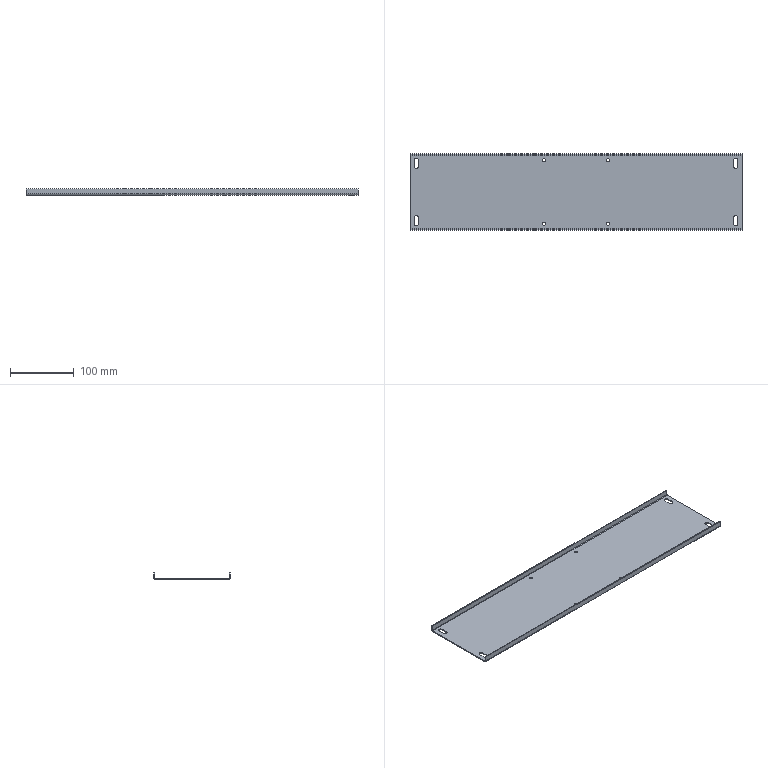Part | STEP file | Guide wheel mechanism revised.sldasm-Part-314 | 1 solid | 46 faces | box 520 x 120 x 10 mm | volume 105158 mm3 | plane 26 | cylinder 20 | commonest cylinder face diameters 5 x8 6.5 x8 1.473 x2 4.473 x2
STEP:
#1=CARTESIAN_POINT('',(-52.5,-50.,-1.5));
#2=VERTEX_POINT('',#1);
#3=CARTESIAN_POINT('',(-47.5,-50.,-1.5));
#4=VERTEX_POINT('',#3);
#5=CARTESIAN_POINT('',(-50.,-50.,-1.5));
#6=DIRECTION('',(0.,0.,1.));
#7=DIRECTION('',(1.,0.,0.));
#8=AXIS2_PLACEMENT_3D('',#5,#6,#7);
#9=CIRCLE('',#8,2.5);
#10=EDGE_CURVE('',#2,#4,#9,.T.);
#11=ORIENTED_EDGE('',*,*,#10,.F.);
#12=CARTESIAN_POINT('',(-52.5,-50.,0.));
#13=VERTEX_POINT('',#12);
#14=CARTESIAN_POINT('',(-52.5,-50.,0.));
#15=DIRECTION('',(0.,0.,1.));
#16=VECTOR('',#15,1000.);
#17=LINE('',#14,#16);
#18=EDGE_CURVE('',#2,#13,#17,.T.);
#19=ORIENTED_EDGE('',*,*,#18,.T.);
#20=CARTESIAN_POINT('',(-47.5,-50.,0.));
#21=VERTEX_POINT('',#20);
#22=CARTESIAN_POINT('',(-50.,-50.,0.));
#23=DIRECTION('',(0.,0.,1.));
#24=DIRECTION('',(1.,0.,0.));
#25=AXIS2_PLACEMENT_3D('',#22,#23,#24);
#26=CIRCLE('',#25,2.5);
#27=EDGE_CURVE('',#13,#21,#26,.T.);
#28=ORIENTED_EDGE('',*,*,#27,.T.);
#29=CARTESIAN_POINT('',(-47.5,-50.,0.));
#30=DIRECTION('',(0.,0.,1.));
#31=VECTOR('',#30,1000.);
#32=LINE('',#29,#31);
#33=EDGE_CURVE('',#4,#21,#32,.T.);
#34=ORIENTED_EDGE('',*,*,#33,.F.);
#35=EDGE_LOOP('',(#11,#19,#28,#34));
#36=FACE_OUTER_BOUND('',#35,.T.);
#37=CARTESIAN_POINT('',(-50.,-50.,0.));
#38=DIRECTION('',(0.,0.,1.));
#39=DIRECTION('',(1.,0.,0.));
#40=AXIS2_PLACEMENT_3D('',#37,#38,#39);
#41=CYLINDRICAL_SURFACE('',#40,2.5);
#42=ADVANCED_FACE('',(#36),#41,.F.);
#43=CARTESIAN_POINT('',(-52.5,50.,-1.5));
#44=VERTEX_POINT('',#43);
#45=CARTESIAN_POINT('',(-47.5,50.,-1.5));
#46=VERTEX_POINT('',#45);
#47=CARTESIAN_POINT('',(-50.,50.,-1.5));
#48=DIRECTION('',(0.,0.,1.));
#49=DIRECTION('',(1.,0.,0.));
#50=AXIS2_PLACEMENT_3D('',#47,#48,#49);
#51=CIRCLE('',#50,2.5);
#52=EDGE_CURVE('',#44,#46,#51,.T.);
#53=ORIENTED_EDGE('',*,*,#52,.F.);
#54=CARTESIAN_POINT('',(-52.5,50.,0.));
#55=VERTEX_POINT('',#54);
#56=CARTESIAN_POINT('',(-52.5,50.,0.));
#57=DIRECTION('',(0.,0.,1.));
#58=VECTOR('',#57,1000.);
#59=LINE('',#56,#58);
#60=EDGE_CURVE('',#44,#55,#59,.T.);
#61=ORIENTED_EDGE('',*,*,#60,.T.);
#62=CARTESIAN_POINT('',(-47.5,50.,0.));
#63=VERTEX_POINT('',#62);
#64=CARTESIAN_POINT('',(-50.,50.,0.));
#65=DIRECTION('',(0.,0.,1.));
#66=DIRECTION('',(1.,0.,0.));
#67=AXIS2_PLACEMENT_3D('',#64,#65,#66);
#68=CIRCLE('',#67,2.5);
#69=EDGE_CURVE('',#55,#63,#68,.T.);
#70=ORIENTED_EDGE('',*,*,#69,.T.);
#71=CARTESIAN_POINT('',(-47.5,50.,0.));
#72=DIRECTION('',(0.,0.,1.));
#73=VECTOR('',#72,1000.);
#74=LINE('',#71,#73);
#75=EDGE_CURVE('',#46,#63,#74,.T.);
#76=ORIENTED_EDGE('',*,*,#75,.F.);
#77=EDGE_LOOP('',(#53,#61,#70,#76));
#78=FACE_OUTER_BOUND('',#77,.T.);
#79=CARTESIAN_POINT('',(-50.,50.,0.));
#80=DIRECTION('',(0.,0.,1.));
#81=DIRECTION('',(1.,0.,0.));
#82=AXIS2_PLACEMENT_3D('',#79,#80,#81);
#83=CYLINDRICAL_SURFACE('',#82,2.5);
#84=ADVANCED_FACE('',(#78),#83,.F.);
#85=CARTESIAN_POINT('',(47.5,-50.,-1.5));
#86=VERTEX_POINT('',#85);
#87=CARTESIAN_POINT('',(52.5,-50.,-1.5));
#88=VERTEX_POINT('',#87);
#89=CARTESIAN_POINT('',(50.,-50.,-1.5));
#90=DIRECTION('',(0.,0.,1.));
#91=DIRECTION('',(1.,0.,0.));
#92=AXIS2_PLACEMENT_3D('',#89,#90,#91);
#93=CIRCLE('',#92,2.5);
#94=EDGE_CURVE('',#86,#88,#93,.T.);
#95=ORIENTED_EDGE('',*,*,#94,.F.);
#96=CARTESIAN_POINT('',(47.5,-50.,0.));
#97=VERTEX_POINT('',#96);
#98=CARTESIAN_POINT('',(47.5,-50.,0.));
#99=DIRECTION('',(0.,0.,1.));
#100=VECTOR('',#99,1000.);
#101=LINE('',#98,#100);
#102=EDGE_CURVE('',#86,#97,#101,.T.);
#103=ORIENTED_EDGE('',*,*,#102,.T.);
#104=CARTESIAN_POINT('',(52.5,-50.,0.));
#105=VERTEX_POINT('',#104);
#106=CARTESIAN_POINT('',(50.,-50.,0.));
#107=DIRECTION('',(0.,0.,1.));
#108=DIRECTION('',(1.,0.,0.));
#109=AXIS2_PLACEMENT_3D('',#106,#107,#108);
#110=CIRCLE('',#109,2.5);
#111=EDGE_CURVE('',#97,#105,#110,.T.);
#112=ORIENTED_EDGE('',*,*,#111,.T.);
#113=CARTESIAN_POINT('',(52.5,-50.,0.));
#114=DIRECTION('',(0.,0.,1.));
#115=VECTOR('',#114,1000.);
#116=LINE('',#113,#115);
#117=EDGE_CURVE('',#88,#105,#116,.T.);
#118=ORIENTED_EDGE('',*,*,#117,.F.);
#119=EDGE_LOOP('',(#95,#103,#112,#118));
#120=FACE_OUTER_BOUND('',#119,.T.);
#121=CARTESIAN_POINT('',(50.,-50.,0.));
#122=DIRECTION('',(0.,0.,1.));
#123=DIRECTION('',(1.,0.,0.));
#124=AXIS2_PLACEMENT_3D('',#121,#122,#123);
#125=CYLINDRICAL_SURFACE('',#124,2.5);
#126=ADVANCED_FACE('',(#120),#125,.F.);
#127=CARTESIAN_POINT('',(47.5,50.,-1.5));
#128=VERTEX_POINT('',#127);
#129=CARTESIAN_POINT('',(52.5,50.,-1.5));
#130=VERTEX_POINT('',#129);
#131=CARTESIAN_POINT('',(50.,50.,-1.5));
#132=DIRECTION('',(0.,0.,1.));
#133=DIRECTION('',(1.,0.,0.));
#134=AXIS2_PLACEMENT_3D('',#131,#132,#133);
#135=CIRCLE('',#134,2.5);
#136=EDGE_CURVE('',#128,#130,#135,.T.);
#137=ORIENTED_EDGE('',*,*,#136,.F.);
#138=CARTESIAN_POINT('',(47.5,50.,0.));
#139=VERTEX_POINT('',#138);
#140=CARTESIAN_POINT('',(47.5,50.,0.));
#141=DIRECTION('',(0.,0.,1.));
#142=VECTOR('',#141,1000.);
#143=LINE('',#140,#142);
#144=EDGE_CURVE('',#128,#139,#143,.T.);
#145=ORIENTED_EDGE('',*,*,#144,.T.);
#146=CARTESIAN_POINT('',(52.5,50.,0.));
#147=VERTEX_POINT('',#146);
#148=CARTESIAN_POINT('',(50.,50.,0.));
#149=DIRECTION('',(0.,0.,1.));
#150=DIRECTION('',(1.,0.,0.));
#151=AXIS2_PLACEMENT_3D('',#148,#149,#150);
#152=CIRCLE('',#151,2.5);
#153=EDGE_CURVE('',#139,#147,#152,.T.);
#154=ORIENTED_EDGE('',*,*,#153,.T.);
#155=CARTESIAN_POINT('',(52.5,50.,0.));
#156=DIRECTION('',(0.,0.,1.));
#157=VECTOR('',#156,1000.);
#158=LINE('',#155,#157);
#159=EDGE_CURVE('',#130,#147,#158,.T.);
#160=ORIENTED_EDGE('',*,*,#159,.F.);
#161=EDGE_LOOP('',(#137,#145,#154,#160));
#162=FACE_OUTER_BOUND('',#161,.T.);
#163=CARTESIAN_POINT('',(50.,50.,0.));
#164=DIRECTION('',(0.,0.,1.));
#165=DIRECTION('',(1.,0.,0.));
#166=AXIS2_PLACEMENT_3D('',#163,#164,#165);
#167=CYLINDRICAL_SURFACE('',#166,2.5);
#168=ADVANCED_FACE('',(#162),#167,.F.);
#169=CARTESIAN_POINT('',(-246.75,50.,-1.5));
#170=VERTEX_POINT('',#169);
#171=CARTESIAN_POINT('',(-246.75,40.,-1.5));
#172=VERTEX_POINT('',#171);
#173=CARTESIAN_POINT('',(-246.75,50.,-1.5));
#174=DIRECTION('',(0.,-1.,0.));
#175=VECTOR('',#174,1000.);
#176=LINE('',#173,#175);
#177=EDGE_CURVE('',#170,#172,#176,.T.);
#178=ORIENTED_EDGE('',*,*,#177,.F.);
#179=CARTESIAN_POINT('',(-253.25,50.,-1.5));
#180=VERTEX_POINT('',#179);
#181=CARTESIAN_POINT('',(-250.,50.,-1.5));
#182=DIRECTION('',(0.,0.,-1.));
#183=DIRECTION('',(-1.,0.,0.));
#184=AXIS2_PLACEMENT_3D('',#181,#182,#183);
#185=CIRCLE('',#184,3.25);
#186=EDGE_CURVE('',#180,#170,#185,.T.);
#187=ORIENTED_EDGE('',*,*,#186,.F.);
#188=CARTESIAN_POINT('',(-253.25,40.,-1.5));
#189=VERTEX_POINT('',#188);
#190=CARTESIAN_POINT('',(-253.25,50.,-1.5));
#191=DIRECTION('',(0.,1.,0.));
#192=VECTOR('',#191,1000.);
#193=LINE('',#190,#192);
#194=EDGE_CURVE('',#189,#180,#193,.T.);
#195=ORIENTED_EDGE('',*,*,#194,.F.);
#196=CARTESIAN_POINT('',(-250.,40.,-1.5));
#197=DIRECTION('',(0.,0.,-1.));
#198=DIRECTION('',(-1.,0.,0.));
#199=AXIS2_PLACEMENT_3D('',#196,#197,#198);
#200=CIRCLE('',#199,3.25);
#201=EDGE_CURVE('',#172,#189,#200,.T.);
#202=ORIENTED_EDGE('',*,*,#201,.F.);
#203=EDGE_LOOP('',(#178,#187,#195,#202));
#204=FACE_BOUND('',#203,.T.);
#205=CARTESIAN_POINT('',(253.25,50.,-1.5));
#206=VERTEX_POINT('',#205);
#207=CARTESIAN_POINT('',(253.25,40.,-1.5));
#208=VERTEX_POINT('',#207);
#209=CARTESIAN_POINT('',(253.25,50.,-1.5));
#210=DIRECTION('',(0.,-1.,0.));
#211=VECTOR('',#210,1000.);
#212=LINE('',#209,#211);
#213=EDGE_CURVE('',#206,#208,#212,.T.);
#214=ORIENTED_EDGE('',*,*,#213,.F.);
#215=CARTESIAN_POINT('',(246.75,50.,-1.5));
#216=VERTEX_POINT('',#215);
#217=CARTESIAN_POINT('',(250.,50.,-1.5));
#218=DIRECTION('',(0.,0.,-1.));
#219=DIRECTION('',(-1.,0.,0.));
#220=AXIS2_PLACEMENT_3D('',#217,#218,#219);
#221=CIRCLE('',#220,3.25);
#222=EDGE_CURVE('',#216,#206,#221,.T.);
#223=ORIENTED_EDGE('',*,*,#222,.F.);
#224=CARTESIAN_POINT('',(246.75,40.,-1.5));
#225=VERTEX_POINT('',#224);
#226=CARTESIAN_POINT('',(246.75,50.,-1.5));
#227=DIRECTION('',(0.,1.,0.));
#228=VECTOR('',#227,1000.);
#229=LINE('',#226,#228);
#230=EDGE_CURVE('',#225,#216,#229,.T.);
#231=ORIENTED_EDGE('',*,*,#230,.F.);
#232=CARTESIAN_POINT('',(250.,40.,-1.5));
#233=DIRECTION('',(0.,0.,-1.));
#234=DIRECTION('',(-1.,0.,0.));
#235=AXIS2_PLACEMENT_3D('',#232,#233,#234);
#236=CIRCLE('',#235,3.25);
#237=EDGE_CURVE('',#208,#225,#236,.T.);
#238=ORIENTED_EDGE('',*,*,#237,.F.);
#239=EDGE_LOOP('',(#214,#223,#231,#238));
#240=FACE_BOUND('',#239,.T.);
#241=CARTESIAN_POINT('',(-50.,-50.,-1.5));
#242=DIRECTION('',(0.,0.,1.));
#243=DIRECTION('',(1.,0.,0.));
#244=AXIS2_PLACEMENT_3D('',#241,#242,#243);
#245=CIRCLE('',#244,2.5);
#246=EDGE_CURVE('',#4,#2,#245,.T.);
#247=ORIENTED_EDGE('',*,*,#246,.T.);
#248=ORIENTED_EDGE('',*,*,#10,.T.);
#249=EDGE_LOOP('',(#247,#248));
#250=FACE_BOUND('',#249,.T.);
#251=CARTESIAN_POINT('',(-50.,50.,-1.5));
#252=DIRECTION('',(0.,0.,1.));
#253=DIRECTION('',(1.,0.,0.));
#254=AXIS2_PLACEMENT_3D('',#251,#252,#253);
#255=CIRCLE('',#254,2.5);
#256=EDGE_CURVE('',#46,#44,#255,.T.);
#257=ORIENTED_EDGE('',*,*,#256,.T.);
#258=ORIENTED_EDGE('',*,*,#52,.T.);
#259=EDGE_LOOP('',(#257,#258));
#260=FACE_BOUND('',#259,.T.);
#261=CARTESIAN_POINT('',(50.,-50.,-1.5));
#262=DIRECTION('',(0.,0.,1.));
#263=DIRECTION('',(1.,0.,0.));
#264=AXIS2_PLACEMENT_3D('',#261,#262,#263);
#265=CIRCLE('',#264,2.5);
#266=EDGE_CURVE('',#88,#86,#265,.T.);
#267=ORIENTED_EDGE('',*,*,#266,.T.);
#268=ORIENTED_EDGE('',*,*,#94,.T.);
#269=EDGE_LOOP('',(#267,#268));
#270=FACE_BOUND('',#269,.T.);
#271=CARTESIAN_POINT('',(50.,50.,-1.5));
#272=DIRECTION('',(0.,0.,1.));
#273=DIRECTION('',(1.,0.,0.));
#274=AXIS2_PLACEMENT_3D('',#271,#272,#273);
#275=CIRCLE('',#274,2.5);
#276=EDGE_CURVE('',#130,#128,#275,.T.);
#277=ORIENTED_EDGE('',*,*,#276,.T.);
#278=ORIENTED_EDGE('',*,*,#136,.T.);
#279=EDGE_LOOP('',(#277,#278));
#280=FACE_BOUND('',#279,.T.);
#281=CARTESIAN_POINT('',(260.,-57.763,-1.5));
#282=VERTEX_POINT('',#281);
#283=CARTESIAN_POINT('',(-260.,-57.763,-1.5));
#284=VERTEX_POINT('',#283);
#285=CARTESIAN_POINT('',(260.,-57.763,-1.5));
#286=DIRECTION('',(-1.,0.,0.));
#287=VECTOR('',#286,1000.);
#288=LINE('',#285,#287);
#289=EDGE_CURVE('',#282,#284,#288,.T.);
#290=ORIENTED_EDGE('',*,*,#289,.T.);
#291=CARTESIAN_POINT('',(-260.,57.763,-1.5));
#292=VERTEX_POINT('',#291);
#293=CARTESIAN_POINT('',(-260.,60.,-1.5));
#294=DIRECTION('',(0.,-1.,0.));
#295=VECTOR('',#294,1000.);
#296=LINE('',#293,#295);
#297=EDGE_CURVE('',#292,#284,#296,.T.);
#298=ORIENTED_EDGE('',*,*,#297,.F.);
#299=CARTESIAN_POINT('',(260.,57.763,-1.5));
#300=VERTEX_POINT('',#299);
#301=CARTESIAN_POINT('',(-260.,57.763,-1.5));
#302=DIRECTION('',(1.,0.,0.));
#303=VECTOR('',#302,1000.);
#304=LINE('',#301,#303);
#305=EDGE_CURVE('',#292,#300,#304,.T.);
#306=ORIENTED_EDGE('',*,*,#305,.T.);
#307=CARTESIAN_POINT('',(260.,60.,-1.5));
#308=DIRECTION('',(0.,1.,0.));
#309=VECTOR('',#308,1000.);
#310=LINE('',#307,#309);
#311=EDGE_CURVE('',#282,#300,#310,.T.);
#312=ORIENTED_EDGE('',*,*,#311,.F.);
#313=EDGE_LOOP('',(#290,#298,#306,#312));
#314=FACE_OUTER_BOUND('',#313,.T.);
#315=CARTESIAN_POINT('',(246.75,-40.,-1.5));
#316=VERTEX_POINT('',#315);
#317=CARTESIAN_POINT('',(253.25,-40.,-1.5));
#318=VERTEX_POINT('',#317);
#319=CARTESIAN_POINT('',(250.,-40.,-1.5));
#320=DIRECTION('',(0.,0.,-1.));
#321=DIRECTION('',(-1.,0.,0.));
#322=AXIS2_PLACEMENT_3D('',#319,#320,#321);
#323=CIRCLE('',#322,3.25);
#324=EDGE_CURVE('',#316,#318,#323,.T.);
#325=ORIENTED_EDGE('',*,*,#324,.F.);
#326=CARTESIAN_POINT('',(246.75,-50.,-1.5));
#327=VERTEX_POINT('',#326);
#328=CARTESIAN_POINT('',(246.75,-40.,-1.5));
#329=DIRECTION('',(0.,1.,0.));
#330=VECTOR('',#329,1000.);
#331=LINE('',#328,#330);
#332=EDGE_CURVE('',#327,#316,#331,.T.);
#333=ORIENTED_EDGE('',*,*,#332,.F.);
#334=CARTESIAN_POINT('',(253.25,-50.,-1.5));
#335=VERTEX_POINT('',#334);
#336=CARTESIAN_POINT('',(250.,-50.,-1.5));
#337=DIRECTION('',(0.,0.,-1.));
#338=DIRECTION('',(-1.,0.,0.));
#339=AXIS2_PLACEMENT_3D('',#336,#337,#338);
#340=CIRCLE('',#339,3.25);
#341=EDGE_CURVE('',#335,#327,#340,.T.);
#342=ORIENTED_EDGE('',*,*,#341,.F.);
#343=CARTESIAN_POINT('',(253.25,-40.,-1.5));
#344=DIRECTION('',(0.,-1.,0.));
#345=VECTOR('',#344,1000.);
#346=LINE('',#343,#345);
#347=EDGE_CURVE('',#318,#335,#346,.T.);
#348=ORIENTED_EDGE('',*,*,#347,.F.);
#349=EDGE_LOOP('',(#325,#333,#342,#348));
#350=FACE_BOUND('',#349,.T.);
#351=CARTESIAN_POINT('',(-253.25,-40.,-1.5));
#352=VERTEX_POINT('',#351);
#353=CARTESIAN_POINT('',(-246.75,-40.,-1.5));
#354=VERTEX_POINT('',#353);
#355=CARTESIAN_POINT('',(-250.,-40.,-1.5));
#356=DIRECTION('',(0.,0.,-1.));
#357=DIRECTION('',(-1.,0.,0.));
#358=AXIS2_PLACEMENT_3D('',#355,#356,#357);
#359=CIRCLE('',#358,3.25);
#360=EDGE_CURVE('',#352,#354,#359,.T.);
#361=ORIENTED_EDGE('',*,*,#360,.F.);
#362=CARTESIAN_POINT('',(-253.25,-50.,-1.5));
#363=VERTEX_POINT('',#362);
#364=CARTESIAN_POINT('',(-253.25,-40.,-1.5));
#365=DIRECTION('',(0.,1.,0.));
#366=VECTOR('',#365,1000.);
#367=LINE('',#364,#366);
#368=EDGE_CURVE('',#363,#352,#367,.T.);
#369=ORIENTED_EDGE('',*,*,#368,.F.);
#370=CARTESIAN_POINT('',(-246.75,-50.,-1.5));
#371=VERTEX_POINT('',#370);
#372=CARTESIAN_POINT('',(-250.,-50.,-1.5));
#373=DIRECTION('',(0.,0.,-1.));
#374=DIRECTION('',(-1.,0.,0.));
#375=AXIS2_PLACEMENT_3D('',#372,#373,#374);
#376=CIRCLE('',#375,3.25);
#377=EDGE_CURVE('',#371,#363,#376,.T.);
#378=ORIENTED_EDGE('',*,*,#377,.F.);
#379=CARTESIAN_POINT('',(-246.75,-40.,-1.5));
#380=DIRECTION('',(0.,-1.,0.));
#381=VECTOR('',#380,1000.);
#382=LINE('',#379,#381);
#383=EDGE_CURVE('',#354,#371,#382,.T.);
#384=ORIENTED_EDGE('',*,*,#383,.F.);
#385=EDGE_LOOP('',(#361,#369,#378,#384));
#386=FACE_BOUND('',#385,.T.);
#387=CARTESIAN_POINT('',(260.,-60.,-1.5));
#388=DIRECTION('',(0.,0.,1.));
#389=DIRECTION('',(1.,0.,0.));
#390=AXIS2_PLACEMENT_3D('',#387,#388,#389);
#391=PLANE('',#390);
#392=ADVANCED_FACE('',(#204,#240,#250,#260,#270,#280,#314,#350,#386),#391,.F.);
#393=CARTESIAN_POINT('',(-253.25,50.,0.));
#394=VERTEX_POINT('',#393);
#395=CARTESIAN_POINT('',(-246.75,50.,0.));
#396=VERTEX_POINT('',#395);
#397=CARTESIAN_POINT('',(-250.,50.,0.));
#398=DIRECTION('',(0.,0.,-1.));
#399=DIRECTION('',(-1.,0.,0.));
#400=AXIS2_PLACEMENT_3D('',#397,#398,#399);
#401=CIRCLE('',#400,3.25);
#402=EDGE_CURVE('',#394,#396,#401,.T.);
#403=ORIENTED_EDGE('',*,*,#402,.T.);
#404=CARTESIAN_POINT('',(-246.75,40.,0.));
#405=VERTEX_POINT('',#404);
#406=CARTESIAN_POINT('',(-246.75,50.,0.));
#407=DIRECTION('',(0.,-1.,0.));
#408=VECTOR('',#407,1000.);
#409=LINE('',#406,#408);
#410=EDGE_CURVE('',#396,#405,#409,.T.);
#411=ORIENTED_EDGE('',*,*,#410,.T.);
#412=CARTESIAN_POINT('',(-253.25,40.,0.));
#413=VERTEX_POINT('',#412);
#414=CARTESIAN_POINT('',(-250.,40.,0.));
#415=DIRECTION('',(0.,0.,-1.));
#416=DIRECTION('',(-1.,0.,0.));
#417=AXIS2_PLACEMENT_3D('',#414,#415,#416);
#418=CIRCLE('',#417,3.25);
#419=EDGE_CURVE('',#405,#413,#418,.T.);
#420=ORIENTED_EDGE('',*,*,#419,.T.);
#421=CARTESIAN_POINT('',(-253.25,50.,0.));
#422=DIRECTION('',(0.,1.,0.));
#423=VECTOR('',#422,1000.);
#424=LINE('',#421,#423);
#425=EDGE_CURVE('',#413,#394,#424,.T.);
#426=ORIENTED_EDGE('',*,*,#425,.T.);
#427=EDGE_LOOP('',(#403,#411,#420,#426));
#428=FACE_BOUND('',#427,.T.);
#429=CARTESIAN_POINT('',(246.75,50.,0.));
#430=VERTEX_POINT('',#429);
#431=CARTESIAN_POINT('',(253.25,50.,0.));
#432=VERTEX_POINT('',#431);
#433=CARTESIAN_POINT('',(250.,50.,0.));
#434=DIRECTION('',(0.,0.,-1.));
#435=DIRECTION('',(-1.,0.,0.));
#436=AXIS2_PLACEMENT_3D('',#433,#434,#435);
#437=CIRCLE('',#436,3.25);
#438=EDGE_CURVE('',#430,#432,#437,.T.);
#439=ORIENTED_EDGE('',*,*,#438,.T.);
#440=CARTESIAN_POINT('',(253.25,40.,0.));
#441=VERTEX_POINT('',#440);
#442=CARTESIAN_POINT('',(253.25,50.,0.));
#443=DIRECTION('',(0.,-1.,0.));
#444=VECTOR('',#443,1000.);
#445=LINE('',#442,#444);
#446=EDGE_CURVE('',#432,#441,#445,.T.);
#447=ORIENTED_EDGE('',*,*,#446,.T.);
#448=CARTESIAN_POINT('',(246.75,40.,0.));
#449=VERTEX_POINT('',#448);
#450=CARTESIAN_POINT('',(250.,40.,0.));
#451=DIRECTION('',(0.,0.,-1.));
#452=DIRECTION('',(-1.,0.,0.));
#453=AXIS2_PLACEMENT_3D('',#450,#451,#452);
#454=CIRCLE('',#453,3.25);
#455=EDGE_CURVE('',#441,#449,#454,.T.);
#456=ORIENTED_EDGE('',*,*,#455,.T.);
#457=CARTESIAN_POINT('',(246.75,50.,0.));
#458=DIRECTION('',(0.,1.,0.));
#459=VECTOR('',#458,1000.);
#460=LINE('',#457,#459);
#461=EDGE_CURVE('',#449,#430,#460,.T.);
#462=ORIENTED_EDGE('',*,*,#461,.T.);
#463=EDGE_LOOP('',(#439,#447,#456,#462));
#464=FACE_BOUND('',#463,.T.);
#465=CARTESIAN_POINT('',(-50.,-50.,0.));
#466=DIRECTION('',(0.,0.,1.));
#467=DIRECTION('',(1.,0.,0.));
#468=AXIS2_PLACEMENT_3D('',#465,#466,#467);
#469=CIRCLE('',#468,2.5);
#470=EDGE_CURVE('',#21,#13,#469,.T.);
#471=ORIENTED_EDGE('',*,*,#470,.F.);
#472=ORIENTED_EDGE('',*,*,#27,.F.);
#473=EDGE_LOOP('',(#471,#472));
#474=FACE_BOUND('',#473,.T.);
#475=CARTESIAN_POINT('',(-50.,50.,0.));
#476=DIRECTION('',(0.,0.,1.));
#477=DIRECTION('',(1.,0.,0.));
#478=AXIS2_PLACEMENT_3D('',#475,#476,#477);
#479=CIRCLE('',#478,2.5);
#480=EDGE_CURVE('',#63,#55,#479,.T.);
#481=ORIENTED_EDGE('',*,*,#480,.F.);
#482=ORIENTED_EDGE('',*,*,#69,.F.);
#483=EDGE_LOOP('',(#481,#482));
#484=FACE_BOUND('',#483,.T.);
#485=CARTESIAN_POINT('',(50.,-50.,0.));
#486=DIRECTION('',(0.,0.,1.));
#487=DIRECTION('',(1.,0.,0.));
#488=AXIS2_PLACEMENT_3D('',#485,#486,#487);
#489=CIRCLE('',#488,2.5);
#490=EDGE_CURVE('',#105,#97,#489,.T.);
#491=ORIENTED_EDGE('',*,*,#490,.F.);
#492=ORIENTED_EDGE('',*,*,#111,.F.);
#493=EDGE_LOOP('',(#491,#492));
#494=FACE_BOUND('',#493,.T.);
#495=CARTESIAN_POINT('',(50.,50.,0.));
#496=DIRECTION('',(0.,0.,1.));
#497=DIRECTION('',(1.,0.,0.));
#498=AXIS2_PLACEMENT_3D('',#495,#496,#497);
#499=CIRCLE('',#498,2.5);
#500=EDGE_CURVE('',#147,#139,#499,.T.);
#501=ORIENTED_EDGE('',*,*,#500,.F.);
#502=ORIENTED_EDGE('',*,*,#153,.F.);
#503=EDGE_LOOP('',(#501,#502));
#504=FACE_BOUND('',#503,.T.);
#505=CARTESIAN_POINT('',(-260.,57.763,0.));
#506=VERTEX_POINT('',#505);
#507=CARTESIAN_POINT('',(-260.,-57.763,0.));
#508=VERTEX_POINT('',#507);
#509=CARTESIAN_POINT('',(-260.,60.,0.));
#510=DIRECTION('',(0.,-1.,0.));
#511=VECTOR('',#510,1000.);
#512=LINE('',#509,#511);
#513=EDGE_CURVE('',#506,#508,#512,.T.);
#514=ORIENTED_EDGE('',*,*,#513,.T.);
#515=CARTESIAN_POINT('',(260.,-57.763,0.));
#516=VERTEX_POINT('',#515);
#517=CARTESIAN_POINT('',(260.,-57.763,0.));
#518=DIRECTION('',(-1.,0.,0.));
#519=VECTOR('',#518,1000.);
#520=LINE('',#517,#519);
#521=EDGE_CURVE('',#516,#508,#520,.T.);
#522=ORIENTED_EDGE('',*,*,#521,.F.);
#523=CARTESIAN_POINT('',(260.,57.763,0.));
#524=VERTEX_POINT('',#523);
#525=CARTESIAN_POINT('',(260.,60.,0.));
#526=DIRECTION('',(0.,1.,0.));
#527=VECTOR('',#526,1000.);
#528=LINE('',#525,#527);
#529=EDGE_CURVE('',#516,#524,#528,.T.);
#530=ORIENTED_EDGE('',*,*,#529,.T.);
#531=CARTESIAN_POINT('',(-260.,57.763,0.));
#532=DIRECTION('',(1.,0.,0.));
#533=VECTOR('',#532,1000.);
#534=LINE('',#531,#533);
#535=EDGE_CURVE('',#506,#524,#534,.T.);
#536=ORIENTED_EDGE('',*,*,#535,.F.);
#537=EDGE_LOOP('',(#514,#522,#530,#536));
#538=FACE_OUTER_BOUND('',#537,.T.);
#539=CARTESIAN_POINT('',(246.75,-40.,0.));
#540=VERTEX_POINT('',#539);
#541=CARTESIAN_POINT('',(253.25,-40.,0.));
#542=VERTEX_POINT('',#541);
#543=CARTESIAN_POINT('',(250.,-40.,0.));
#544=DIRECTION('',(0.,0.,-1.));
#545=DIRECTION('',(-1.,0.,0.));
#546=AXIS2_PLACEMENT_3D('',#543,#544,#545);
#547=CIRCLE('',#546,3.25);
#548=EDGE_CURVE('',#540,#542,#547,.T.);
#549=ORIENTED_EDGE('',*,*,#548,.T.);
#550=CARTESIAN_POINT('',(253.25,-50.,0.));
#551=VERTEX_POINT('',#550);
#552=CARTESIAN_POINT('',(253.25,-40.,0.));
#553=DIRECTION('',(0.,-1.,0.));
#554=VECTOR('',#553,1000.);
#555=LINE('',#552,#554);
#556=EDGE_CURVE('',#542,#551,#555,.T.);
#557=ORIENTED_EDGE('',*,*,#556,.T.);
#558=CARTESIAN_POINT('',(246.75,-50.,0.));
#559=VERTEX_POINT('',#558);
#560=CARTESIAN_POINT('',(250.,-50.,0.));
#561=DIRECTION('',(0.,0.,-1.));
#562=DIRECTION('',(-1.,0.,0.));
#563=AXIS2_PLACEMENT_3D('',#560,#561,#562);
#564=CIRCLE('',#563,3.25);
#565=EDGE_CURVE('',#551,#559,#564,.T.);
#566=ORIENTED_EDGE('',*,*,#565,.T.);
#567=CARTESIAN_POINT('',(246.75,-40.,0.));
#568=DIRECTION('',(0.,1.,0.));
#569=VECTOR('',#568,1000.);
#570=LINE('',#567,#569);
#571=EDGE_CURVE('',#559,#540,#570,.T.);
#572=ORIENTED_EDGE('',*,*,#571,.T.);
#573=EDGE_LOOP('',(#549,#557,#566,#572));
#574=FACE_BOUND('',#573,.T.);
#575=CARTESIAN_POINT('',(-253.25,-40.,0.));
#576=VERTEX_POINT('',#575);
#577=CARTESIAN_POINT('',(-246.75,-40.,0.));
#578=VERTEX_POINT('',#577);
#579=CARTESIAN_POINT('',(-250.,-40.,0.));
#580=DIRECTION('',(0.,0.,-1.));
#581=DIRECTION('',(-1.,0.,0.));
#582=AXIS2_PLACEMENT_3D('',#579,#580,#581);
#583=CIRCLE('',#582,3.25);
#584=EDGE_CURVE('',#576,#578,#583,.T.);
#585=ORIENTED_EDGE('',*,*,#584,.T.);
#586=CARTESIAN_POINT('',(-246.75,-50.,0.));
#587=VERTEX_POINT('',#586);
#588=CARTESIAN_POINT('',(-246.75,-40.,0.));
#589=DIRECTION('',(0.,-1.,0.));
#590=VECTOR('',#589,1000.);
#591=LINE('',#588,#590);
#592=EDGE_CURVE('',#578,#587,#591,.T.);
#593=ORIENTED_EDGE('',*,*,#592,.T.);
#594=CARTESIAN_POINT('',(-253.25,-50.,0.));
#595=VERTEX_POINT('',#594);
#596=CARTESIAN_POINT('',(-250.,-50.,0.));
#597=DIRECTION('',(0.,0.,-1.));
#598=DIRECTION('',(-1.,0.,0.));
#599=AXIS2_PLACEMENT_3D('',#596,#597,#598);
#600=CIRCLE('',#599,3.25);
#601=EDGE_CURVE('',#587,#595,#600,.T.);
#602=ORIENTED_EDGE('',*,*,#601,.T.);
#603=CARTESIAN_POINT('',(-253.25,-40.,0.));
#604=DIRECTION('',(0.,1.,0.));
#605=VECTOR('',#604,1000.);
#606=LINE('',#603,#605);
#607=EDGE_CURVE('',#595,#576,#606,.T.);
#608=ORIENTED_EDGE('',*,*,#607,.T.);
#609=EDGE_LOOP('',(#585,#593,#602,#608));
#610=FACE_BOUND('',#609,.T.);
#611=CARTESIAN_POINT('',(260.,-60.,0.));
#612=DIRECTION('',(0.,0.,1.));
#613=DIRECTION('',(1.,0.,0.));
#614=AXIS2_PLACEMENT_3D('',#611,#612,#613);
#615=PLANE('',#614);
#616=ADVANCED_FACE('',(#428,#464,#474,#484,#494,#504,#538,#574,#610),#615,.T.);
#617=ORIENTED_EDGE('',*,*,#529,.F.);
#618=CARTESIAN_POINT('',(260.,-57.763,0.));
#619=DIRECTION('',(0.,0.,-1.));
#620=VECTOR('',#619,1000.);
#621=LINE('',#618,#620);
#622=EDGE_CURVE('',#516,#282,#621,.T.);
#623=ORIENTED_EDGE('',*,*,#622,.T.);
#624=ORIENTED_EDGE('',*,*,#311,.T.);
#625=CARTESIAN_POINT('',(260.,57.763,0.));
#626=DIRECTION('',(0.,0.,-1.));
#627=VECTOR('',#626,1000.);
#628=LINE('',#625,#627);
#629=EDGE_CURVE('',#524,#300,#628,.T.);
#630=ORIENTED_EDGE('',*,*,#629,.F.);
#631=EDGE_LOOP('',(#617,#623,#624,#630));
#632=FACE_OUTER_BOUND('',#631,.T.);
#633=CARTESIAN_POINT('',(260.,60.,-1.5));
#634=DIRECTION('',(1.,0.,0.));
#635=DIRECTION('',(0.,1.,0.));
#636=AXIS2_PLACEMENT_3D('',#633,#634,#635);
#637=PLANE('',#636);
#638=ADVANCED_FACE('',(#632),#637,.T.);
#639=CARTESIAN_POINT('',(-260.,-57.763,0.));
#640=DIRECTION('',(0.,0.,-1.));
#641=VECTOR('',#640,1000.);
#642=LINE('',#639,#641);
#643=EDGE_CURVE('',#508,#284,#642,.T.);
#644=ORIENTED_EDGE('',*,*,#643,.F.);
#645=ORIENTED_EDGE('',*,*,#513,.F.);
#646=CARTESIAN_POINT('',(-260.,57.763,0.));
#647=DIRECTION('',(0.,0.,-1.));
#648=VECTOR('',#647,1000.);
#649=LINE('',#646,#648);
#650=EDGE_CURVE('',#506,#292,#649,.T.);
#651=ORIENTED_EDGE('',*,*,#650,.T.);
#652=ORIENTED_EDGE('',*,*,#297,.T.);
#653=EDGE_LOOP('',(#644,#645,#651,#652));
#654=FACE_OUTER_BOUND('',#653,.T.);
#655=CARTESIAN_POINT('',(-260.,60.,-1.5));
#656=DIRECTION('',(-1.,0.,0.));
#657=DIRECTION('',(0.,-1.,0.));
#658=AXIS2_PLACEMENT_3D('',#655,#656,#657);
#659=PLANE('',#658);
#660=ADVANCED_FACE('',(#654),#659,.T.);
#661=ORIENTED_EDGE('',*,*,#144,.F.);
#662=ORIENTED_EDGE('',*,*,#276,.F.);
#663=ORIENTED_EDGE('',*,*,#159,.T.);
#664=ORIENTED_EDGE('',*,*,#500,.T.);
#665=EDGE_LOOP('',(#661,#662,#663,#664));
#666=FACE_OUTER_BOUND('',#665,.T.);
#667=CARTESIAN_POINT('',(50.,50.,0.));
#668=DIRECTION('',(0.,0.,1.));
#669=DIRECTION('',(1.,0.,0.));
#670=AXIS2_PLACEMENT_3D('',#667,#668,#669);
#671=CYLINDRICAL_SURFACE('',#670,2.5);
#672=ADVANCED_FACE('',(#666),#671,.F.);
#673=ORIENTED_EDGE('',*,*,#102,.F.);
#674=ORIENTED_EDGE('',*,*,#266,.F.);
#675=ORIENTED_EDGE('',*,*,#117,.T.);
#676=ORIENTED_EDGE('',*,*,#490,.T.);
#677=EDGE_LOOP('',(#673,#674,#675,#676));
#678=FACE_OUTER_BOUND('',#677,.T.);
#679=CARTESIAN_POINT('',(50.,-50.,0.));
#680=DIRECTION('',(0.,0.,1.));
#681=DIRECTION('',(1.,0.,0.));
#682=AXIS2_PLACEMENT_3D('',#679,#680,#681);
#683=CYLINDRICAL_SURFACE('',#682,2.5);
#684=ADVANCED_FACE('',(#678),#683,.F.);
#685=ORIENTED_EDGE('',*,*,#60,.F.);
#686=ORIENTED_EDGE('',*,*,#256,.F.);
#687=ORIENTED_EDGE('',*,*,#75,.T.);
#688=ORIENTED_EDGE('',*,*,#480,.T.);
#689=EDGE_LOOP('',(#685,#686,#687,#688));
#690=FACE_OUTER_BOUND('',#689,.T.);
#691=CARTESIAN_POINT('',(-50.,50.,0.));
#692=DIRECTION('',(0.,0.,1.));
#693=DIRECTION('',(1.,0.,0.));
#694=AXIS2_PLACEMENT_3D('',#691,#692,#693);
#695=CYLINDRICAL_SURFACE('',#694,2.5);
#696=ADVANCED_FACE('',(#690),#695,.F.);
#697=ORIENTED_EDGE('',*,*,#18,.F.);
#698=ORIENTED_EDGE('',*,*,#246,.F.);
#699=ORIENTED_EDGE('',*,*,#33,.T.);
#700=ORIENTED_EDGE('',*,*,#470,.T.);
#701=EDGE_LOOP('',(#697,#698,#699,#700));
#702=FACE_OUTER_BOUND('',#701,.T.);
#703=CARTESIAN_POINT('',(-50.,-50.,0.));
#704=DIRECTION('',(0.,0.,1.));
#705=DIRECTION('',(1.,0.,0.));
#706=AXIS2_PLACEMENT_3D('',#703,#704,#705);
#707=CYLINDRICAL_SURFACE('',#706,2.5);
#708=ADVANCED_FACE('',(#702),#707,.F.);
#709=CARTESIAN_POINT('',(260.,58.5,0.7366));
#710=VERTEX_POINT('',#709);
#711=CARTESIAN_POINT('',(260.,60.,0.7366));
#712=VERTEX_POINT('',#711);
#713=CARTESIAN_POINT('',(260.,60.,0.7366));
#714=DIRECTION('',(0.,1.,0.));
#715=VECTOR('',#714,1000.);
#716=LINE('',#713,#715);
#717=EDGE_CURVE('',#710,#712,#716,.T.);
#718=ORIENTED_EDGE('',*,*,#717,.F.);
#719=CARTESIAN_POINT('',(260.,57.763,0.7366));
#720=DIRECTION('',(1.,0.,0.));
#721=DIRECTION('',(0.,0.,1.));
#722=AXIS2_PLACEMENT_3D('',#719,#720,#721);
#723=CIRCLE('',#722,0.7366);
#724=EDGE_CURVE('',#524,#710,#723,.T.);
#725=ORIENTED_EDGE('',*,*,#724,.F.);
#726=ORIENTED_EDGE('',*,*,#629,.T.);
#727=CARTESIAN_POINT('',(260.,57.763,0.7366));
#728=DIRECTION('',(1.,0.,0.));
#729=DIRECTION('',(0.,0.,1.));
#730=AXIS2_PLACEMENT_3D('',#727,#728,#729);
#731=CIRCLE('',#730,2.237);
#732=EDGE_CURVE('',#300,#712,#731,.T.);
#733=ORIENTED_EDGE('',*,*,#732,.T.);
#734=EDGE_LOOP('',(#718,#725,#726,#733));
#735=FACE_OUTER_BOUND('',#734,.T.);
#736=CARTESIAN_POINT('',(260.,57.763,0.7366));
#737=DIRECTION('',(1.,0.,0.));
#738=DIRECTION('',(0.,0.,-1.));
#739=AXIS2_PLACEMENT_3D('',#736,#737,#738);
#740=PLANE('',#739);
#741=ADVANCED_FACE('',(#735),#740,.T.);
#742=ORIENTED_EDGE('',*,*,#305,.F.);
#743=CARTESIAN_POINT('',(-260.,60.,0.7366));
#744=VERTEX_POINT('',#743);
#745=CARTESIAN_POINT('',(-260.,57.763,0.7366));
#746=DIRECTION('',(-1.,0.,0.));
#747=DIRECTION('',(0.,0.,1.));
#748=AXIS2_PLACEMENT_3D('',#745,#746,#747);
#749=CIRCLE('',#748,2.237);
#750=EDGE_CURVE('',#744,#292,#749,.T.);
#751=ORIENTED_EDGE('',*,*,#750,.F.);
#752=CARTESIAN_POINT('',(260.,60.,0.7366));
#753=DIRECTION('',(1.,0.,0.));
#754=VECTOR('',#753,1000.);
#755=LINE('',#752,#754);
#756=EDGE_CURVE('',#744,#712,#755,.T.);
#757=ORIENTED_EDGE('',*,*,#756,.T.);
#758=ORIENTED_EDGE('',*,*,#732,.F.);
#759=EDGE_LOOP('',(#742,#751,#757,#758));
#760=FACE_OUTER_BOUND('',#759,.T.);
#761=CARTESIAN_POINT('',(-260.,57.763,0.7366));
#762=DIRECTION('',(-1.,0.,0.));
#763=DIRECTION('',(0.,1.,0.));
#764=AXIS2_PLACEMENT_3D('',#761,#762,#763);
#765=CYLINDRICAL_SURFACE('',#764,2.237);
#766=ADVANCED_FACE('',(#760),#765,.T.);
#767=CARTESIAN_POINT('',(-260.,58.5,0.7366));
#768=VERTEX_POINT('',#767);
#769=CARTESIAN_POINT('',(-260.,57.763,0.7366));
#770=DIRECTION('',(-1.,0.,0.));
#771=DIRECTION('',(0.,0.,1.));
#772=AXIS2_PLACEMENT_3D('',#769,#770,#771);
#773=CIRCLE('',#772,0.7366);
#774=EDGE_CURVE('',#768,#506,#773,.T.);
#775=ORIENTED_EDGE('',*,*,#774,.F.);
#776=CARTESIAN_POINT('',(-260.,58.5,0.7366));
#777=DIRECTION('',(0.,1.,0.));
#778=VECTOR('',#777,1000.);
#779=LINE('',#776,#778);
#780=EDGE_CURVE('',#768,#744,#779,.T.);
#781=ORIENTED_EDGE('',*,*,#780,.T.);
#782=ORIENTED_EDGE('',*,*,#750,.T.);
#783=ORIENTED_EDGE('',*,*,#650,.F.);
#784=EDGE_LOOP('',(#775,#781,#782,#783));
#785=FACE_OUTER_BOUND('',#784,.T.);
#786=CARTESIAN_POINT('',(-260.,57.763,0.7366));
#787=DIRECTION('',(1.,0.,0.));
#788=DIRECTION('',(0.,0.,-1.));
#789=AXIS2_PLACEMENT_3D('',#786,#787,#788);
#790=PLANE('',#789);
#791=ADVANCED_FACE('',(#785),#790,.F.);
#792=ORIENTED_EDGE('',*,*,#535,.T.);
#793=ORIENTED_EDGE('',*,*,#724,.T.);
#794=CARTESIAN_POINT('',(260.,58.5,0.7366));
#795=DIRECTION('',(-1.,0.,0.));
#796=VECTOR('',#795,1000.);
#797=LINE('',#794,#796);
#798=EDGE_CURVE('',#710,#768,#797,.T.);
#799=ORIENTED_EDGE('',*,*,#798,.T.);
#800=ORIENTED_EDGE('',*,*,#774,.T.);
#801=EDGE_LOOP('',(#792,#793,#799,#800));
#802=FACE_OUTER_BOUND('',#801,.T.);
#803=CARTESIAN_POINT('',(-260.,57.763,0.7366));
#804=DIRECTION('',(-1.,0.,0.));
#805=DIRECTION('',(0.,1.,0.));
#806=AXIS2_PLACEMENT_3D('',#803,#804,#805);
#807=CYLINDRICAL_SURFACE('',#806,0.7366);
#808=ADVANCED_FACE('',(#802),#807,.F.);
#809=ORIENTED_EDGE('',*,*,#780,.F.);
#810=CARTESIAN_POINT('',(-260.,58.5,8.5));
#811=VERTEX_POINT('',#810);
#812=CARTESIAN_POINT('',(-260.,58.5,8.5));
#813=DIRECTION('',(0.,0.,1.));
#814=VECTOR('',#813,1000.);
#815=LINE('',#812,#814);
#816=EDGE_CURVE('',#768,#811,#815,.T.);
#817=ORIENTED_EDGE('',*,*,#816,.T.);
#818=CARTESIAN_POINT('',(-260.,60.,8.5));
#819=VERTEX_POINT('',#818);
#820=CARTESIAN_POINT('',(-260.,60.,8.5));
#821=DIRECTION('',(0.,-1.,0.));
#822=VECTOR('',#821,1000.);
#823=LINE('',#820,#822);
#824=EDGE_CURVE('',#819,#811,#823,.T.);
#825=ORIENTED_EDGE('',*,*,#824,.F.);
#826=CARTESIAN_POINT('',(-260.,60.,0.));
#827=DIRECTION('',(0.,0.,1.));
#828=VECTOR('',#827,1000.);
#829=LINE('',#826,#828);
#830=EDGE_CURVE('',#744,#819,#829,.T.);
#831=ORIENTED_EDGE('',*,*,#830,.F.);
#832=EDGE_LOOP('',(#809,#817,#825,#831));
#833=FACE_OUTER_BOUND('',#832,.T.);
#834=CARTESIAN_POINT('',(-260.,60.,8.5));
#835=DIRECTION('',(1.,0.,0.));
#836=DIRECTION('',(0.,0.,-1.));
#837=AXIS2_PLACEMENT_3D('',#834,#835,#836);
#838=PLANE('',#837);
#839=ADVANCED_FACE('',(#833),#838,.F.);
#840=ORIENTED_EDGE('',*,*,#717,.T.);
#841=CARTESIAN_POINT('',(260.,60.,8.5));
#842=VERTEX_POINT('',#841);
#843=CARTESIAN_POINT('',(260.,60.,0.));
#844=DIRECTION('',(0.,0.,-1.));
#845=VECTOR('',#844,1000.);
#846=LINE('',#843,#845);
#847=EDGE_CURVE('',#842,#712,#846,.T.);
#848=ORIENTED_EDGE('',*,*,#847,.F.);
#849=CARTESIAN_POINT('',(260.,58.5,8.5));
#850=VERTEX_POINT('',#849);
#851=CARTESIAN_POINT('',(260.,60.,8.5));
#852=DIRECTION('',(0.,-1.,0.));
#853=VECTOR('',#852,1000.);
#854=LINE('',#851,#853);
#855=EDGE_CURVE('',#842,#850,#854,.T.);
#856=ORIENTED_EDGE('',*,*,#855,.T.);
#857=CARTESIAN_POINT('',(260.,58.5,0.));
#858=DIRECTION('',(0.,0.,-1.));
#859=VECTOR('',#858,1000.);
#860=LINE('',#857,#859);
#861=EDGE_CURVE('',#850,#710,#860,.T.);
#862=ORIENTED_EDGE('',*,*,#861,.T.);
#863=EDGE_LOOP('',(#840,#848,#856,#862));
#864=FACE_OUTER_BOUND('',#863,.T.);
#865=CARTESIAN_POINT('',(260.,60.,0.));
#866=DIRECTION('',(-1.,0.,0.));
#867=DIRECTION('',(0.,0.,1.));
#868=AXIS2_PLACEMENT_3D('',#865,#866,#867);
#869=PLANE('',#868);
#870=ADVANCED_FACE('',(#864),#869,.F.);
#871=ORIENTED_EDGE('',*,*,#756,.F.);
#872=ORIENTED_EDGE('',*,*,#830,.T.);
#873=CARTESIAN_POINT('',(-260.,60.,8.5));
#874=DIRECTION('',(1.,0.,0.));
#875=VECTOR('',#874,1000.);
#876=LINE('',#873,#875);
#877=EDGE_CURVE('',#819,#842,#876,.T.);
#878=ORIENTED_EDGE('',*,*,#877,.T.);
#879=ORIENTED_EDGE('',*,*,#847,.T.);
#880=EDGE_LOOP('',(#871,#872,#878,#879));
#881=FACE_OUTER_BOUND('',#880,.T.);
#882=CARTESIAN_POINT('',(-260.,60.,0.));
#883=DIRECTION('',(0.,-1.,0.));
#884=DIRECTION('',(0.,0.,-1.));
#885=AXIS2_PLACEMENT_3D('',#882,#883,#884);
#886=PLANE('',#885);
#887=ADVANCED_FACE('',(#881),#886,.F.);
#888=ORIENTED_EDGE('',*,*,#816,.F.);
#889=ORIENTED_EDGE('',*,*,#798,.F.);
#890=ORIENTED_EDGE('',*,*,#861,.F.);
#891=CARTESIAN_POINT('',(260.,58.5,8.5));
#892=DIRECTION('',(1.,0.,0.));
#893=VECTOR('',#892,1000.);
#894=LINE('',#891,#893);
#895=EDGE_CURVE('',#811,#850,#894,.T.);
#896=ORIENTED_EDGE('',*,*,#895,.F.);
#897=EDGE_LOOP('',(#888,#889,#890,#896));
#898=FACE_OUTER_BOUND('',#897,.T.);
#899=CARTESIAN_POINT('',(-260.,58.5,0.));
#900=DIRECTION('',(0.,-1.,0.));
#901=DIRECTION('',(0.,0.,-1.));
#902=AXIS2_PLACEMENT_3D('',#899,#900,#901);
#903=PLANE('',#902);
#904=ADVANCED_FACE('',(#898),#903,.T.);
#905=ORIENTED_EDGE('',*,*,#895,.T.);
#906=ORIENTED_EDGE('',*,*,#855,.F.);
#907=ORIENTED_EDGE('',*,*,#877,.F.);
#908=ORIENTED_EDGE('',*,*,#824,.T.);
#909=EDGE_LOOP('',(#905,#906,#907,#908));
#910=FACE_OUTER_BOUND('',#909,.T.);
#911=CARTESIAN_POINT('',(260.,60.,8.5));
#912=DIRECTION('',(0.,0.,-1.));
#913=DIRECTION('',(0.,1.,0.));
#914=AXIS2_PLACEMENT_3D('',#911,#912,#913);
#915=PLANE('',#914);
#916=ADVANCED_FACE('',(#910),#915,.F.);
#917=CARTESIAN_POINT('',(-260.,-58.5,0.7366));
#918=VERTEX_POINT('',#917);
#919=CARTESIAN_POINT('',(-260.,-60.,0.7366));
#920=VERTEX_POINT('',#919);
#921=CARTESIAN_POINT('',(-260.,-60.,0.7366));
#922=DIRECTION('',(0.,-1.,0.));
#923=VECTOR('',#922,1000.);
#924=LINE('',#921,#923);
#925=EDGE_CURVE('',#918,#920,#924,.T.);
#926=ORIENTED_EDGE('',*,*,#925,.F.);
#927=CARTESIAN_POINT('',(-260.,-57.763,0.7366));
#928=DIRECTION('',(-1.,0.,0.));
#929=DIRECTION('',(0.,0.,-1.));
#930=AXIS2_PLACEMENT_3D('',#927,#928,#929);
#931=CIRCLE('',#930,0.7366);
#932=EDGE_CURVE('',#508,#918,#931,.T.);
#933=ORIENTED_EDGE('',*,*,#932,.F.);
#934=ORIENTED_EDGE('',*,*,#643,.T.);
#935=CARTESIAN_POINT('',(-260.,-57.763,0.7366));
#936=DIRECTION('',(-1.,0.,0.));
#937=DIRECTION('',(0.,0.,-1.));
#938=AXIS2_PLACEMENT_3D('',#935,#936,#937);
#939=CIRCLE('',#938,2.237);
#940=EDGE_CURVE('',#284,#920,#939,.T.);
#941=ORIENTED_EDGE('',*,*,#940,.T.);
#942=EDGE_LOOP('',(#926,#933,#934,#941));
#943=FACE_OUTER_BOUND('',#942,.T.);
#944=CARTESIAN_POINT('',(-260.,-57.763,0.7366));
#945=DIRECTION('',(-1.,0.,0.));
#946=DIRECTION('',(0.,0.,1.));
#947=AXIS2_PLACEMENT_3D('',#944,#945,#946);
#948=PLANE('',#947);
#949=ADVANCED_FACE('',(#943),#948,.T.);
#950=ORIENTED_EDGE('',*,*,#289,.F.);
#951=CARTESIAN_POINT('',(260.,-60.,0.7366));
#952=VERTEX_POINT('',#951);
#953=CARTESIAN_POINT('',(260.,-57.763,0.7366));
#954=DIRECTION('',(1.,0.,0.));
#955=DIRECTION('',(0.,0.,-1.));
#956=AXIS2_PLACEMENT_3D('',#953,#954,#955);
#957=CIRCLE('',#956,2.237);
#958=EDGE_CURVE('',#952,#282,#957,.T.);
#959=ORIENTED_EDGE('',*,*,#958,.F.);
#960=CARTESIAN_POINT('',(260.,-60.,0.7366));
#961=DIRECTION('',(1.,0.,0.));
#962=VECTOR('',#961,1000.);
#963=LINE('',#960,#962);
#964=EDGE_CURVE('',#920,#952,#963,.T.);
#965=ORIENTED_EDGE('',*,*,#964,.F.);
#966=ORIENTED_EDGE('',*,*,#940,.F.);
#967=EDGE_LOOP('',(#950,#959,#965,#966));
#968=FACE_OUTER_BOUND('',#967,.T.);
#969=CARTESIAN_POINT('',(260.,-57.763,0.7366));
#970=DIRECTION('',(1.,0.,0.));
#971=DIRECTION('',(0.,-1.,0.));
#972=AXIS2_PLACEMENT_3D('',#969,#970,#971);
#973=CYLINDRICAL_SURFACE('',#972,2.237);
#974=ADVANCED_FACE('',(#968),#973,.T.);
#975=CARTESIAN_POINT('',(260.,-58.5,0.7366));
#976=VERTEX_POINT('',#975);
#977=CARTESIAN_POINT('',(260.,-57.763,0.7366));
#978=DIRECTION('',(1.,0.,0.));
#979=DIRECTION('',(0.,0.,-1.));
#980=AXIS2_PLACEMENT_3D('',#977,#978,#979);
#981=CIRCLE('',#980,0.7366);
#982=EDGE_CURVE('',#976,#516,#981,.T.);
#983=ORIENTED_EDGE('',*,*,#982,.F.);
#984=CARTESIAN_POINT('',(260.,-58.5,0.7366));
#985=DIRECTION('',(0.,-1.,0.));
#986=VECTOR('',#985,1000.);
#987=LINE('',#984,#986);
#988=EDGE_CURVE('',#976,#952,#987,.T.);
#989=ORIENTED_EDGE('',*,*,#988,.T.);
#990=ORIENTED_EDGE('',*,*,#958,.T.);
#991=ORIENTED_EDGE('',*,*,#622,.F.);
#992=EDGE_LOOP('',(#983,#989,#990,#991));
#993=FACE_OUTER_BOUND('',#992,.T.);
#994=CARTESIAN_POINT('',(260.,-57.763,0.7366));
#995=DIRECTION('',(-1.,0.,0.));
#996=DIRECTION('',(0.,0.,1.));
#997=AXIS2_PLACEMENT_3D('',#994,#995,#996);
#998=PLANE('',#997);
#999=ADVANCED_FACE('',(#993),#998,.F.);
#1000=ORIENTED_EDGE('',*,*,#521,.T.);
#1001=ORIENTED_EDGE('',*,*,#932,.T.);
#1002=CARTESIAN_POINT('',(-260.,-58.5,0.7366));
#1003=DIRECTION('',(1.,0.,0.));
#1004=VECTOR('',#1003,1000.);
#1005=LINE('',#1002,#1004);
#1006=EDGE_CURVE('',#918,#976,#1005,.T.);
#1007=ORIENTED_EDGE('',*,*,#1006,.T.);
#1008=ORIENTED_EDGE('',*,*,#982,.T.);
#1009=EDGE_LOOP('',(#1000,#1001,#1007,#1008));
#1010=FACE_OUTER_BOUND('',#1009,.T.);
#1011=CARTESIAN_POINT('',(260.,-57.763,0.7366));
#1012=DIRECTION('',(1.,0.,0.));
#1013=DIRECTION('',(0.,-1.,0.));
#1014=AXIS2_PLACEMENT_3D('',#1011,#1012,#1013);
#1015=CYLINDRICAL_SURFACE('',#1014,0.7366);
#1016=ADVANCED_FACE('',(#1010),#1015,.F.);
#1017=ORIENTED_EDGE('',*,*,#988,.F.);
#1018=CARTESIAN_POINT('',(260.,-58.5,8.5));
#1019=VERTEX_POINT('',#1018);
#1020=CARTESIAN_POINT('',(260.,-58.5,0.));
#1021=DIRECTION('',(0.,0.,1.));
#1022=VECTOR('',#1021,1000.);
#1023=LINE('',#1020,#1022);
#1024=EDGE_CURVE('',#976,#1019,#1023,.T.);
#1025=ORIENTED_EDGE('',*,*,#1024,.T.);
#1026=CARTESIAN_POINT('',(260.,-60.,8.5));
#1027=VERTEX_POINT('',#1026);
#1028=CARTESIAN_POINT('',(260.,-60.,8.5));
#1029=DIRECTION('',(0.,1.,0.));
#1030=VECTOR('',#1029,1000.);
#1031=LINE('',#1028,#1030);
#1032=EDGE_CURVE('',#1027,#1019,#1031,.T.);
#1033=ORIENTED_EDGE('',*,*,#1032,.F.);
#1034=CARTESIAN_POINT('',(260.,-60.,0.));
#1035=DIRECTION('',(0.,0.,1.));
#1036=VECTOR('',#1035,1000.);
#1037=LINE('',#1034,#1036);
#1038=EDGE_CURVE('',#952,#1027,#1037,.T.);
#1039=ORIENTED_EDGE('',*,*,#1038,.F.);
#1040=EDGE_LOOP('',(#1017,#1025,#1033,#1039));
#1041=FACE_OUTER_BOUND('',#1040,.T.);
#1042=CARTESIAN_POINT('',(260.,-60.,0.));
#1043=DIRECTION('',(-1.,0.,0.));
#1044=DIRECTION('',(0.,0.,1.));
#1045=AXIS2_PLACEMENT_3D('',#1042,#1043,#1044);
#1046=PLANE('',#1045);
#1047=ADVANCED_FACE('',(#1041),#1046,.F.);
#1048=ORIENTED_EDGE('',*,*,#925,.T.);
#1049=CARTESIAN_POINT('',(-260.,-60.,8.5));
#1050=VERTEX_POINT('',#1049);
#1051=CARTESIAN_POINT('',(-260.,-60.,0.));
#1052=DIRECTION('',(0.,0.,-1.));
#1053=VECTOR('',#1052,1000.);
#1054=LINE('',#1051,#1053);
#1055=EDGE_CURVE('',#1050,#920,#1054,.T.);
#1056=ORIENTED_EDGE('',*,*,#1055,.F.);
#1057=CARTESIAN_POINT('',(-260.,-58.5,8.5));
#1058=VERTEX_POINT('',#1057);
#1059=CARTESIAN_POINT('',(-260.,-60.,8.5));
#1060=DIRECTION('',(0.,1.,0.));
#1061=VECTOR('',#1060,1000.);
#1062=LINE('',#1059,#1061);
#1063=EDGE_CURVE('',#1050,#1058,#1062,.T.);
#1064=ORIENTED_EDGE('',*,*,#1063,.T.);
#1065=CARTESIAN_POINT('',(-260.,-58.5,8.5));
#1066=DIRECTION('',(0.,0.,-1.));
#1067=VECTOR('',#1066,1000.);
#1068=LINE('',#1065,#1067);
#1069=EDGE_CURVE('',#1058,#918,#1068,.T.);
#1070=ORIENTED_EDGE('',*,*,#1069,.T.);
#1071=EDGE_LOOP('',(#1048,#1056,#1064,#1070));
#1072=FACE_OUTER_BOUND('',#1071,.T.);
#1073=CARTESIAN_POINT('',(-260.,-60.,8.5));
#1074=DIRECTION('',(1.,0.,0.));
#1075=DIRECTION('',(0.,0.,-1.));
#1076=AXIS2_PLACEMENT_3D('',#1073,#1074,#1075);
#1077=PLANE('',#1076);
#1078=ADVANCED_FACE('',(#1072),#1077,.F.);
#1079=ORIENTED_EDGE('',*,*,#1055,.T.);
#1080=ORIENTED_EDGE('',*,*,#964,.T.);
#1081=ORIENTED_EDGE('',*,*,#1038,.T.);
#1082=CARTESIAN_POINT('',(260.,-60.,8.5));
#1083=DIRECTION('',(-1.,0.,0.));
#1084=VECTOR('',#1083,1000.);
#1085=LINE('',#1082,#1084);
#1086=EDGE_CURVE('',#1027,#1050,#1085,.T.);
#1087=ORIENTED_EDGE('',*,*,#1086,.T.);
#1088=EDGE_LOOP('',(#1079,#1080,#1081,#1087));
#1089=FACE_OUTER_BOUND('',#1088,.T.);
#1090=CARTESIAN_POINT('',(260.,-60.,0.));
#1091=DIRECTION('',(0.,-1.,0.));
#1092=DIRECTION('',(0.,0.,-1.));
#1093=AXIS2_PLACEMENT_3D('',#1090,#1091,#1092);
#1094=PLANE('',#1093);
#1095=ADVANCED_FACE('',(#1089),#1094,.T.);
#1096=ORIENTED_EDGE('',*,*,#1006,.F.);
#1097=ORIENTED_EDGE('',*,*,#1069,.F.);
#1098=CARTESIAN_POINT('',(260.,-58.5,8.5));
#1099=DIRECTION('',(-1.,0.,0.));
#1100=VECTOR('',#1099,1000.);
#1101=LINE('',#1098,#1100);
#1102=EDGE_CURVE('',#1019,#1058,#1101,.T.);
#1103=ORIENTED_EDGE('',*,*,#1102,.F.);
#1104=ORIENTED_EDGE('',*,*,#1024,.F.);
#1105=EDGE_LOOP('',(#1096,#1097,#1103,#1104));
#1106=FACE_OUTER_BOUND('',#1105,.T.);
#1107=CARTESIAN_POINT('',(260.,-58.5,0.));
#1108=DIRECTION('',(0.,-1.,0.));
#1109=DIRECTION('',(0.,0.,-1.));
#1110=AXIS2_PLACEMENT_3D('',#1107,#1108,#1109);
#1111=PLANE('',#1110);
#1112=ADVANCED_FACE('',(#1106),#1111,.F.);
#1113=ORIENTED_EDGE('',*,*,#1102,.T.);
#1114=ORIENTED_EDGE('',*,*,#1063,.F.);
#1115=ORIENTED_EDGE('',*,*,#1086,.F.);
#1116=ORIENTED_EDGE('',*,*,#1032,.T.);
#1117=EDGE_LOOP('',(#1113,#1114,#1115,#1116));
#1118=FACE_OUTER_BOUND('',#1117,.T.);
#1119=CARTESIAN_POINT('',(260.,-60.,8.5));
#1120=DIRECTION('',(0.,0.,-1.));
#1121=DIRECTION('',(0.,1.,0.));
#1122=AXIS2_PLACEMENT_3D('',#1119,#1120,#1121);
#1123=PLANE('',#1122);
#1124=ADVANCED_FACE('',(#1118),#1123,.F.);
#1125=ORIENTED_EDGE('',*,*,#222,.T.);
#1126=CARTESIAN_POINT('',(253.25,50.,0.));
#1127=DIRECTION('',(0.,0.,-1.));
#1128=VECTOR('',#1127,1000.);
#1129=LINE('',#1126,#1128);
#1130=EDGE_CURVE('',#432,#206,#1129,.T.);
#1131=ORIENTED_EDGE('',*,*,#1130,.F.);
#1132=ORIENTED_EDGE('',*,*,#438,.F.);
#1133=CARTESIAN_POINT('',(246.75,50.,0.));
#1134=DIRECTION('',(0.,0.,-1.));
#1135=VECTOR('',#1134,1000.);
#1136=LINE('',#1133,#1135);
#1137=EDGE_CURVE('',#430,#216,#1136,.T.);
#1138=ORIENTED_EDGE('',*,*,#1137,.T.);
#1139=EDGE_LOOP('',(#1125,#1131,#1132,#1138));
#1140=FACE_OUTER_BOUND('',#1139,.T.);
#1141=CARTESIAN_POINT('',(250.,50.,0.));
#1142=DIRECTION('',(0.,0.,-1.));
#1143=DIRECTION('',(-1.,0.,0.));
#1144=AXIS2_PLACEMENT_3D('',#1141,#1142,#1143);
#1145=CYLINDRICAL_SURFACE('',#1144,3.25);
#1146=ADVANCED_FACE('',(#1140),#1145,.F.);
#1147=ORIENTED_EDGE('',*,*,#230,.T.);
#1148=ORIENTED_EDGE('',*,*,#1137,.F.);
#1149=ORIENTED_EDGE('',*,*,#461,.F.);
#1150=CARTESIAN_POINT('',(246.75,40.,0.));
#1151=DIRECTION('',(0.,0.,-1.));
#1152=VECTOR('',#1151,1000.);
#1153=LINE('',#1150,#1152);
#1154=EDGE_CURVE('',#449,#225,#1153,.T.);
#1155=ORIENTED_EDGE('',*,*,#1154,.T.);
#1156=EDGE_LOOP('',(#1147,#1148,#1149,#1155));
#1157=FACE_OUTER_BOUND('',#1156,.T.);
#1158=CARTESIAN_POINT('',(246.75,50.,0.));
#1159=DIRECTION('',(-1.,0.,0.));
#1160=DIRECTION('',(0.,0.,1.));
#1161=AXIS2_PLACEMENT_3D('',#1158,#1159,#1160);
#1162=PLANE('',#1161);
#1163=ADVANCED_FACE('',(#1157),#1162,.F.);
#1164=ORIENTED_EDGE('',*,*,#237,.T.);
#1165=ORIENTED_EDGE('',*,*,#1154,.F.);
#1166=ORIENTED_EDGE('',*,*,#455,.F.);
#1167=CARTESIAN_POINT('',(253.25,40.,0.));
#1168=DIRECTION('',(0.,0.,-1.));
#1169=VECTOR('',#1168,1000.);
#1170=LINE('',#1167,#1169);
#1171=EDGE_CURVE('',#441,#208,#1170,.T.);
#1172=ORIENTED_EDGE('',*,*,#1171,.T.);
#1173=EDGE_LOOP('',(#1164,#1165,#1166,#1172));
#1174=FACE_OUTER_BOUND('',#1173,.T.);
#1175=CARTESIAN_POINT('',(250.,40.,0.));
#1176=DIRECTION('',(0.,0.,-1.));
#1177=DIRECTION('',(-1.,0.,0.));
#1178=AXIS2_PLACEMENT_3D('',#1175,#1176,#1177);
#1179=CYLINDRICAL_SURFACE('',#1178,3.25);
#1180=ADVANCED_FACE('',(#1174),#1179,.F.);
#1181=ORIENTED_EDGE('',*,*,#213,.T.);
#1182=ORIENTED_EDGE('',*,*,#1171,.F.);
#1183=ORIENTED_EDGE('',*,*,#446,.F.);
#1184=ORIENTED_EDGE('',*,*,#1130,.T.);
#1185=EDGE_LOOP('',(#1181,#1182,#1183,#1184));
#1186=FACE_OUTER_BOUND('',#1185,.T.);
#1187=CARTESIAN_POINT('',(253.25,50.,0.));
#1188=DIRECTION('',(1.,0.,0.));
#1189=DIRECTION('',(0.,0.,-1.));
#1190=AXIS2_PLACEMENT_3D('',#1187,#1188,#1189);
#1191=PLANE('',#1190);
#1192=ADVANCED_FACE('',(#1186),#1191,.F.);
#1193=ORIENTED_EDGE('',*,*,#177,.T.);
#1194=CARTESIAN_POINT('',(-246.75,40.,0.));
#1195=DIRECTION('',(0.,0.,-1.));
#1196=VECTOR('',#1195,1000.);
#1197=LINE('',#1194,#1196);
#1198=EDGE_CURVE('',#405,#172,#1197,.T.);
#1199=ORIENTED_EDGE('',*,*,#1198,.F.);
#1200=ORIENTED_EDGE('',*,*,#410,.F.);
#1201=CARTESIAN_POINT('',(-246.75,50.,0.));
#1202=DIRECTION('',(0.,0.,-1.));
#1203=VECTOR('',#1202,1000.);
#1204=LINE('',#1201,#1203);
#1205=EDGE_CURVE('',#396,#170,#1204,.T.);
#1206=ORIENTED_EDGE('',*,*,#1205,.T.);
#1207=EDGE_LOOP('',(#1193,#1199,#1200,#1206));
#1208=FACE_OUTER_BOUND('',#1207,.T.);
#1209=CARTESIAN_POINT('',(-246.75,50.,0.));
#1210=DIRECTION('',(1.,0.,0.));
#1211=DIRECTION('',(0.,0.,-1.));
#1212=AXIS2_PLACEMENT_3D('',#1209,#1210,#1211);
#1213=PLANE('',#1212);
#1214=ADVANCED_FACE('',(#1208),#1213,.F.);
#1215=ORIENTED_EDGE('',*,*,#201,.T.);
#1216=CARTESIAN_POINT('',(-253.25,40.,0.));
#1217=DIRECTION('',(0.,0.,-1.));
#1218=VECTOR('',#1217,1000.);
#1219=LINE('',#1216,#1218);
#1220=EDGE_CURVE('',#413,#189,#1219,.T.);
#1221=ORIENTED_EDGE('',*,*,#1220,.F.);
#1222=ORIENTED_EDGE('',*,*,#419,.F.);
#1223=ORIENTED_EDGE('',*,*,#1198,.T.);
#1224=EDGE_LOOP('',(#1215,#1221,#1222,#1223));
#1225=FACE_OUTER_BOUND('',#1224,.T.);
#1226=CARTESIAN_POINT('',(-250.,40.,0.));
#1227=DIRECTION('',(0.,0.,-1.));
#1228=DIRECTION('',(-1.,0.,0.));
#1229=AXIS2_PLACEMENT_3D('',#1226,#1227,#1228);
#1230=CYLINDRICAL_SURFACE('',#1229,3.25);
#1231=ADVANCED_FACE('',(#1225),#1230,.F.);
#1232=ORIENTED_EDGE('',*,*,#194,.T.);
#1233=CARTESIAN_POINT('',(-253.25,50.,0.));
#1234=DIRECTION('',(0.,0.,-1.));
#1235=VECTOR('',#1234,1000.);
#1236=LINE('',#1233,#1235);
#1237=EDGE_CURVE('',#394,#180,#1236,.T.);
#1238=ORIENTED_EDGE('',*,*,#1237,.F.);
#1239=ORIENTED_EDGE('',*,*,#425,.F.);
#1240=ORIENTED_EDGE('',*,*,#1220,.T.);
#1241=EDGE_LOOP('',(#1232,#1238,#1239,#1240));
#1242=FACE_OUTER_BOUND('',#1241,.T.);
#1243=CARTESIAN_POINT('',(-253.25,50.,0.));
#1244=DIRECTION('',(-1.,0.,0.));
#1245=DIRECTION('',(0.,0.,1.));
#1246=AXIS2_PLACEMENT_3D('',#1243,#1244,#1245);
#1247=PLANE('',#1246);
#1248=ADVANCED_FACE('',(#1242),#1247,.F.);
#1249=ORIENTED_EDGE('',*,*,#186,.T.);
#1250=ORIENTED_EDGE('',*,*,#1205,.F.);
#1251=ORIENTED_EDGE('',*,*,#402,.F.);
#1252=ORIENTED_EDGE('',*,*,#1237,.T.);
#1253=EDGE_LOOP('',(#1249,#1250,#1251,#1252));
#1254=FACE_OUTER_BOUND('',#1253,.T.);
#1255=CARTESIAN_POINT('',(-250.,50.,0.));
#1256=DIRECTION('',(0.,0.,-1.));
#1257=DIRECTION('',(-1.,0.,0.));
#1258=AXIS2_PLACEMENT_3D('',#1255,#1256,#1257);
#1259=CYLINDRICAL_SURFACE('',#1258,3.25);
#1260=ADVANCED_FACE('',(#1254),#1259,.F.);
#1261=ORIENTED_EDGE('',*,*,#347,.T.);
#1262=CARTESIAN_POINT('',(253.25,-50.,0.));
#1263=DIRECTION('',(0.,0.,-1.));
#1264=VECTOR('',#1263,1000.);
#1265=LINE('',#1262,#1264);
#1266=EDGE_CURVE('',#551,#335,#1265,.T.);
#1267=ORIENTED_EDGE('',*,*,#1266,.F.);
#1268=ORIENTED_EDGE('',*,*,#556,.F.);
#1269=CARTESIAN_POINT('',(253.25,-40.,0.));
#1270=DIRECTION('',(0.,0.,-1.));
#1271=VECTOR('',#1270,1000.);
#1272=LINE('',#1269,#1271);
#1273=EDGE_CURVE('',#542,#318,#1272,.T.);
#1274=ORIENTED_EDGE('',*,*,#1273,.T.);
#1275=EDGE_LOOP('',(#1261,#1267,#1268,#1274));
#1276=FACE_OUTER_BOUND('',#1275,.T.);
#1277=CARTESIAN_POINT('',(253.25,-40.,0.));
#1278=DIRECTION('',(1.,0.,0.));
#1279=DIRECTION('',(0.,0.,-1.));
#1280=AXIS2_PLACEMENT_3D('',#1277,#1278,#1279);
#1281=PLANE('',#1280);
#1282=ADVANCED_FACE('',(#1276),#1281,.F.);
#1283=ORIENTED_EDGE('',*,*,#341,.T.);
#1284=CARTESIAN_POINT('',(246.75,-50.,0.));
#1285=DIRECTION('',(0.,0.,-1.));
#1286=VECTOR('',#1285,1000.);
#1287=LINE('',#1284,#1286);
#1288=EDGE_CURVE('',#559,#327,#1287,.T.);
#1289=ORIENTED_EDGE('',*,*,#1288,.F.);
#1290=ORIENTED_EDGE('',*,*,#565,.F.);
#1291=ORIENTED_EDGE('',*,*,#1266,.T.);
#1292=EDGE_LOOP('',(#1283,#1289,#1290,#1291));
#1293=FACE_OUTER_BOUND('',#1292,.T.);
#1294=CARTESIAN_POINT('',(250.,-50.,0.));
#1295=DIRECTION('',(0.,0.,-1.));
#1296=DIRECTION('',(-1.,0.,0.));
#1297=AXIS2_PLACEMENT_3D('',#1294,#1295,#1296);
#1298=CYLINDRICAL_SURFACE('',#1297,3.25);
#1299=ADVANCED_FACE('',(#1293),#1298,.F.);
#1300=ORIENTED_EDGE('',*,*,#332,.T.);
#1301=CARTESIAN_POINT('',(246.75,-40.,0.));
#1302=DIRECTION('',(0.,0.,-1.));
#1303=VECTOR('',#1302,1000.);
#1304=LINE('',#1301,#1303);
#1305=EDGE_CURVE('',#540,#316,#1304,.T.);
#1306=ORIENTED_EDGE('',*,*,#1305,.F.);
#1307=ORIENTED_EDGE('',*,*,#571,.F.);
#1308=ORIENTED_EDGE('',*,*,#1288,.T.);
#1309=EDGE_LOOP('',(#1300,#1306,#1307,#1308));
#1310=FACE_OUTER_BOUND('',#1309,.T.);
#1311=CARTESIAN_POINT('',(246.75,-40.,0.));
#1312=DIRECTION('',(-1.,0.,0.));
#1313=DIRECTION('',(0.,0.,1.));
#1314=AXIS2_PLACEMENT_3D('',#1311,#1312,#1313);
#1315=PLANE('',#1314);
#1316=ADVANCED_FACE('',(#1310),#1315,.F.);
#1317=ORIENTED_EDGE('',*,*,#324,.T.);
#1318=ORIENTED_EDGE('',*,*,#1273,.F.);
#1319=ORIENTED_EDGE('',*,*,#548,.F.);
#1320=ORIENTED_EDGE('',*,*,#1305,.T.);
#1321=EDGE_LOOP('',(#1317,#1318,#1319,#1320));
#1322=FACE_OUTER_BOUND('',#1321,.T.);
#1323=CARTESIAN_POINT('',(250.,-40.,0.));
#1324=DIRECTION('',(0.,0.,-1.));
#1325=DIRECTION('',(-1.,0.,0.));
#1326=AXIS2_PLACEMENT_3D('',#1323,#1324,#1325);
#1327=CYLINDRICAL_SURFACE('',#1326,3.25);
#1328=ADVANCED_FACE('',(#1322),#1327,.F.);
#1329=ORIENTED_EDGE('',*,*,#383,.T.);
#1330=CARTESIAN_POINT('',(-246.75,-50.,0.));
#1331=DIRECTION('',(0.,0.,-1.));
#1332=VECTOR('',#1331,1000.);
#1333=LINE('',#1330,#1332);
#1334=EDGE_CURVE('',#587,#371,#1333,.T.);
#1335=ORIENTED_EDGE('',*,*,#1334,.F.);
#1336=ORIENTED_EDGE('',*,*,#592,.F.);
#1337=CARTESIAN_POINT('',(-246.75,-40.,0.));
#1338=DIRECTION('',(0.,0.,-1.));
#1339=VECTOR('',#1338,1000.);
#1340=LINE('',#1337,#1339);
#1341=EDGE_CURVE('',#578,#354,#1340,.T.);
#1342=ORIENTED_EDGE('',*,*,#1341,.T.);
#1343=EDGE_LOOP('',(#1329,#1335,#1336,#1342));
#1344=FACE_OUTER_BOUND('',#1343,.T.);
#1345=CARTESIAN_POINT('',(-246.75,-40.,0.));
#1346=DIRECTION('',(1.,0.,0.));
#1347=DIRECTION('',(0.,0.,-1.));
#1348=AXIS2_PLACEMENT_3D('',#1345,#1346,#1347);
#1349=PLANE('',#1348);
#1350=ADVANCED_FACE('',(#1344),#1349,.F.);
#1351=ORIENTED_EDGE('',*,*,#377,.T.);
#1352=CARTESIAN_POINT('',(-253.25,-50.,0.));
#1353=DIRECTION('',(0.,0.,-1.));
#1354=VECTOR('',#1353,1000.);
#1355=LINE('',#1352,#1354);
#1356=EDGE_CURVE('',#595,#363,#1355,.T.);
#1357=ORIENTED_EDGE('',*,*,#1356,.F.);
#1358=ORIENTED_EDGE('',*,*,#601,.F.);
#1359=ORIENTED_EDGE('',*,*,#1334,.T.);
#1360=EDGE_LOOP('',(#1351,#1357,#1358,#1359));
#1361=FACE_OUTER_BOUND('',#1360,.T.);
#1362=CARTESIAN_POINT('',(-250.,-50.,0.));
#1363=DIRECTION('',(0.,0.,-1.));
#1364=DIRECTION('',(-1.,0.,0.));
#1365=AXIS2_PLACEMENT_3D('',#1362,#1363,#1364);
#1366=CYLINDRICAL_SURFACE('',#1365,3.25);
#1367=ADVANCED_FACE('',(#1361),#1366,.F.);
#1368=ORIENTED_EDGE('',*,*,#368,.T.);
#1369=CARTESIAN_POINT('',(-253.25,-40.,0.));
#1370=DIRECTION('',(0.,0.,-1.));
#1371=VECTOR('',#1370,1000.);
#1372=LINE('',#1369,#1371);
#1373=EDGE_CURVE('',#576,#352,#1372,.T.);
#1374=ORIENTED_EDGE('',*,*,#1373,.F.);
#1375=ORIENTED_EDGE('',*,*,#607,.F.);
#1376=ORIENTED_EDGE('',*,*,#1356,.T.);
#1377=EDGE_LOOP('',(#1368,#1374,#1375,#1376));
#1378=FACE_OUTER_BOUND('',#1377,.T.);
#1379=CARTESIAN_POINT('',(-253.25,-40.,0.));
#1380=DIRECTION('',(-1.,0.,0.));
#1381=DIRECTION('',(0.,0.,1.));
#1382=AXIS2_PLACEMENT_3D('',#1379,#1380,#1381);
#1383=PLANE('',#1382);
#1384=ADVANCED_FACE('',(#1378),#1383,.F.);
#1385=ORIENTED_EDGE('',*,*,#360,.T.);
#1386=ORIENTED_EDGE('',*,*,#1341,.F.);
#1387=ORIENTED_EDGE('',*,*,#584,.F.);
#1388=ORIENTED_EDGE('',*,*,#1373,.T.);
#1389=EDGE_LOOP('',(#1385,#1386,#1387,#1388));
#1390=FACE_OUTER_BOUND('',#1389,.T.);
#1391=CARTESIAN_POINT('',(-250.,-40.,0.));
#1392=DIRECTION('',(0.,0.,-1.));
#1393=DIRECTION('',(-1.,0.,0.));
#1394=AXIS2_PLACEMENT_3D('',#1391,#1392,#1393);
#1395=CYLINDRICAL_SURFACE('',#1394,3.25);
#1396=ADVANCED_FACE('',(#1390),#1395,.F.);
#1397=CLOSED_SHELL('',(#42,#84,#126,#168,#392,#616,#638,#660,#672,#684,#696,#708,#741,#766,#791,#808,#839,#870,#887,#904,#916,#949,#974,#999,#1016,#1047,#1078,#1095,#1112,#1124,#1146,#1163,#1180,#1192,#1214,#1231,#1248,#1260,#1282,#1299,#1316,#1328,#1350,#1367,#1384,#1396));
#1398=MANIFOLD_SOLID_BREP('',#1397);
#1399=CARTESIAN_POINT('',(0.,0.,0.));
#1400=DIRECTION('',(0.,0.,1.));
#1401=DIRECTION('',(1.,0.,0.));
#1402=AXIS2_PLACEMENT_3D('',#1399,#1400,#1401);
#1403=(LENGTH_UNIT()NAMED_UNIT(*)SI_UNIT(.MILLI.,.METRE.));
#1404=UNCERTAINTY_MEASURE_WITH_UNIT(LENGTH_MEASURE(0.00001),#1403,'','');
#1405=(NAMED_UNIT(*)PLANE_ANGLE_UNIT()SI_UNIT($,.RADIAN.));
#1406=(NAMED_UNIT(*)SI_UNIT($,.STERADIAN.)SOLID_ANGLE_UNIT());
#1407=(GEOMETRIC_REPRESENTATION_CONTEXT(3)GLOBAL_UNCERTAINTY_ASSIGNED_CONTEXT((#1404))GLOBAL_UNIT_ASSIGNED_CONTEXT((#1403,#1405,#1406))REPRESENTATION_CONTEXT('',''));
#1408=ADVANCED_BREP_SHAPE_REPRESENTATION('',(#1398,#1402),#1407);